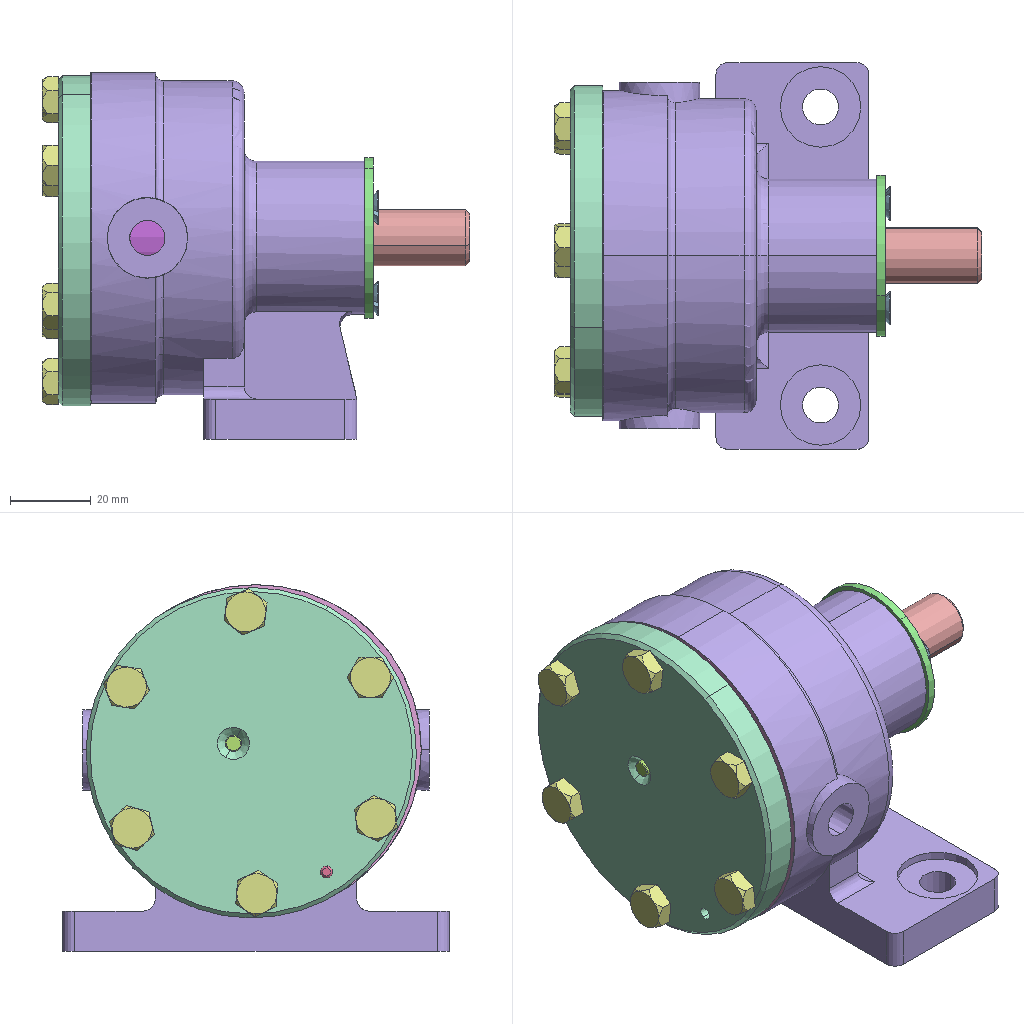Assembly | SolidWorks | 13 different items | 20 placed | box 106 x 96 x 91 mm
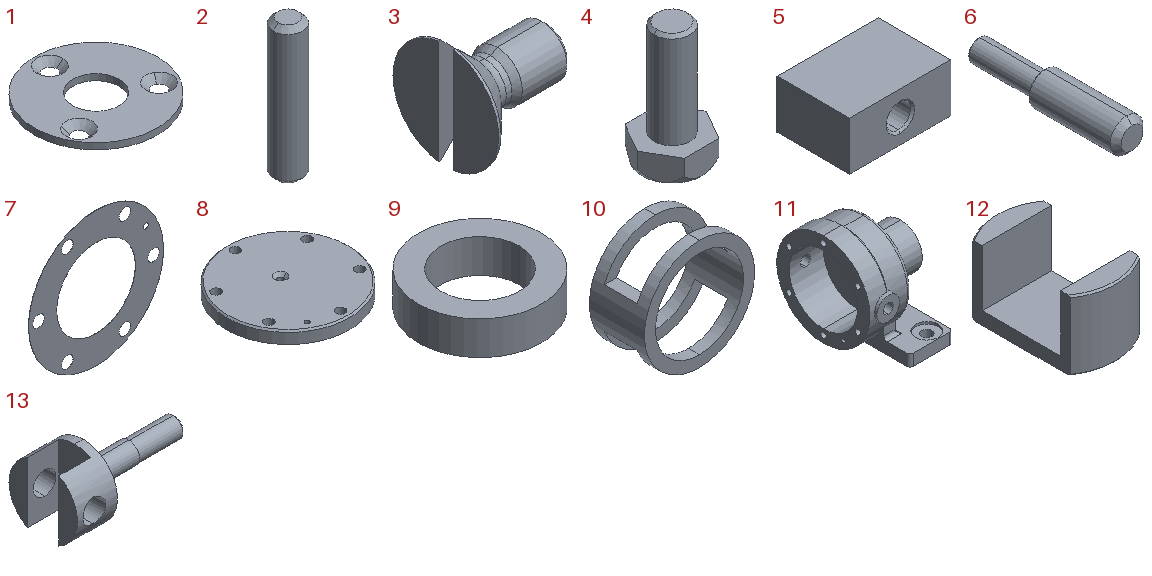Parts list (item | quantity | size | volume | features):
1 | x1 | 40 x 40 x 2 mm | 1954 mm3 | features CirPattern 1, RevCut 1, Revolution 1
2 | x1 | 3 x 3 x 14 mm | 96.866 mm3 | features Chamfer 1, Extrusion 1
3 | x3 | 8 x 8.4 x 8.314 mm | 133.872 mm3 | features Chamfer 1, Cut 1, LPattern 1, RevCut 1, Revolution 1
4 | x6 | 11.547 x 10 x 20 mm | 793.318 mm3 | features ICE 2, Chamfer 1, Extrusion 1
5 | x1 | 25 x 18 x 12 mm | 4886 mm3 | features Chamfer 1, Extrusion 1, ICE 1
6 | x1 | 6 x 28 x 6 mm | 594.197 mm3 | features Revolution 1
7 | x1 | 82 x 0.1 x 82 mm | 323.348 mm3 | features Extrusion 1
8 | x1 | 82 x 82 x 10 mm | 44167 mm3 | features Chamfer 2, ICE 1, Revolution 1
9 | x1 | 22 x 22 x 6 mm | 1357 mm3 | features Revolution 1
10 | x1 | 60 x 30 x 60 mm | 17111 mm3 | features Extrusion 1, ICE 1
11 | x1 | 68 x 96 x 91 mm | 170738 mm3 | features ICE 7, HoleWzd 4, Revolution 2, Chamfer 1, Fillet 1, Rib 1
12 | x1 | 22 x 38 x 22 mm | 7394 mm3 | features Chamfer 1, Extrusion 1, ICE 1
13 | x1 | 92 x 48 x 48 mm | 33624 mm3 | features ICE 2, Chamfer 1, RevCut 1, Revolution 1
Mates (type | each side: item.copy, entity, surface, feature):
Coincident | 9.1 face plane Revolve1 | 11.1 face plane Cut-Extrude3
Concentric | 11.1 face cylinder M4 Tapped Hole1 | 1.1 edge | 2 times
Coincident | 11.1 face plane Revolve1 | 1.1 face plane Revolve1
Concentric | 11.1 face cylinder M4 Tapped Hole1 | 3.1 face cylinder Base-Revolve
Concentric | 11.1 face cylinder M4 Tapped Hole1 | 3.2 edge
Concentric | 11.1 face cylinder M4 Tapped Hole1 | 3.3 face cylinder Base-Revolve
Coincident | 1.1 face plane Revolve1 | 3.1 face plane Cut-Extrude1
Coincident | 1.1 face plane Revolve1 | 3.2 face plane Cut-Extrude1
Coincident | 1.1 face plane Revolve1 | 3.3 face plane Cut-Extrude1
Concentric | 13.1 face cylinder Revolve1 | 10.1 face cylinder Boss-Extrude1
Coincident | 10.1 face plane Boss-Extrude1 | 11.1 face plane Cut-Extrude1
Concentric | 9.1 face cylinder Revolve1 | 10.1 face cylinder Boss-Extrude1
Concentric | 9.1 face cylinder Revolve1 | 11.1 face cylinder Cut-Extrude3
Coincident | 13.1 vertex | 12.1 vertex | 2 times
Parallel | 13.1 face plane Cut-Extrude1 | 12.1 face plane Boss-Extrude1
Coincident | 5.1 face plane Boss-Extrude1 | 12.1 face plane Cut-Extrude1 | 2 times
Width | 13.1 face plane Cut-Extrude1 | 13.1 face plane Cut-Extrude1 | 5.1 face plane Boss-Extrude1 | 5.1 face plane Boss-Extrude1
Coincident | 13.1 face plane Revolve1 | 11.1 face plane Cut-Extrude1
Concentric | 7.1 edge | 11.1 face cylinder Cut-Extrude4
Coincident | 7.1 face plane Boss-Extrude1 | 11.1 face plane Revolve1
Concentric | 7.1 edge | 11.1 face cone M6 Tapped Hole1
Concentric | 5.1 face cylinder Cut-Extrude1 | 8.1 face cylinder Cut-Extrude1
Concentric | 11.1 face cylinder Cut-Extrude4 | 8.1 face cylinder Cut-Extrude1
Coincident | 7.1 face plane Boss-Extrude1 | 8.1 face plane Revolve1
Concentric | 5.1 face cylinder Cut-Extrude1 | 6.1 face cylinder Revolve1
Coincident | 6.1 face plane Revolve1 | 12.1 face plane Cut-Extrude1
Concentric | 2.1 face cylinder Boss-Extrude1 | 8.1 face cylinder Cut-Extrude1
Coincident | 11.1 edge | 2.1 edge
Concentric | 4.1 face cylinder Boss-Extrude2 | 8.1 face cylinder Cut-Extrude1
Coincident | 4.1 face plane Boss-Extrude1 | 8.1 face plane Revolve1
Concentric | 4.2 face cylinder Boss-Extrude2 | 8.1 face cylinder Cut-Extrude1
Coincident | 4.2 face plane Boss-Extrude1 | 8.1 face plane Revolve1
Concentric | 4.3 face cylinder Boss-Extrude2 | 8.1 face cylinder Cut-Extrude1
Concentric | 4.4 face cylinder Boss-Extrude2 | 8.1 face cylinder Cut-Extrude1
Concentric | 4.5 face cylinder Boss-Extrude2 | 8.1 face cylinder Cut-Extrude1
Concentric | 4.6 face cylinder Boss-Extrude2 | 8.1 face cylinder Cut-Extrude1
Coincident | 8.1 face plane Revolve1 | 4.3 face plane Boss-Extrude1
Coincident | 4.6 face plane Boss-Extrude1 | 8.1 face plane Revolve1
Coincident | 4.5 face plane Boss-Extrude1 | 8.1 face plane Revolve1
Coincident | 4.4 face plane Boss-Extrude1 | 8.1 face plane Revolve1